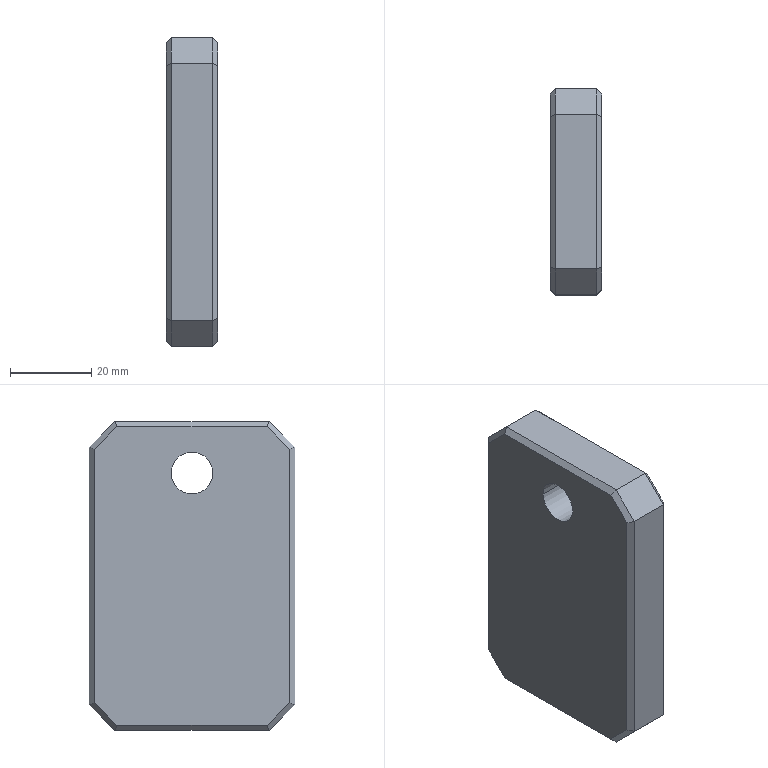Part | STEP file | 4-20.sldasm-Part-60 | 1 solid | 28 faces | box 12.7 x 50.8 x 76.2 mm | volume 46694 mm3 | plane 26 | cylinder 2 | commonest cylinder face diameters 10.317 x2
STEP:
#1=CARTESIAN_POINT('',(237.7,-154.229,175.9));
#2=VERTEX_POINT('',#1);
#3=CARTESIAN_POINT('',(237.7,-143.911,175.9));
#4=VERTEX_POINT('',#3);
#5=CARTESIAN_POINT('',(237.7,-149.07,175.9));
#6=DIRECTION('',(1.,0.,0.));
#7=DIRECTION('',(0.,0.,-1.));
#8=AXIS2_PLACEMENT_3D('',#5,#6,#7);
#9=CIRCLE('',#8,5.159);
#10=EDGE_CURVE('',#2,#4,#9,.T.);
#11=ORIENTED_EDGE('',*,*,#10,.T.);
#12=CARTESIAN_POINT('',(225.,-143.911,175.9));
#13=VERTEX_POINT('',#12);
#14=CARTESIAN_POINT('',(244.05,-143.911,175.9));
#15=DIRECTION('',(-1.,0.,0.));
#16=VECTOR('',#15,1000.);
#17=LINE('',#14,#16);
#18=EDGE_CURVE('',#4,#13,#17,.T.);
#19=ORIENTED_EDGE('',*,*,#18,.T.);
#20=CARTESIAN_POINT('',(225.,-154.229,175.9));
#21=VERTEX_POINT('',#20);
#22=CARTESIAN_POINT('',(225.,-149.07,175.9));
#23=DIRECTION('',(-1.,0.,0.));
#24=DIRECTION('',(0.,-1.,0.));
#25=AXIS2_PLACEMENT_3D('',#22,#23,#24);
#26=CIRCLE('',#25,5.159);
#27=EDGE_CURVE('',#13,#21,#26,.T.);
#28=ORIENTED_EDGE('',*,*,#27,.T.);
#29=CARTESIAN_POINT('',(244.05,-154.229,175.9));
#30=DIRECTION('',(-1.,0.,0.));
#31=VECTOR('',#30,1000.);
#32=LINE('',#29,#31);
#33=EDGE_CURVE('',#2,#21,#32,.T.);
#34=ORIENTED_EDGE('',*,*,#33,.F.);
#35=EDGE_LOOP('',(#11,#19,#28,#34));
#36=FACE_OUTER_BOUND('',#35,.T.);
#37=CARTESIAN_POINT('',(244.05,-149.07,175.9));
#38=DIRECTION('',(-1.,0.,0.));
#39=DIRECTION('',(0.,-1.,0.));
#40=AXIS2_PLACEMENT_3D('',#37,#38,#39);
#41=CYLINDRICAL_SURFACE('',#40,5.159);
#42=ADVANCED_FACE('',(#36),#41,.F.);
#43=CARTESIAN_POINT('',(237.7,-124.94,119.276));
#44=VERTEX_POINT('',#43);
#45=CARTESIAN_POINT('',(237.7,-124.94,181.724));
#46=VERTEX_POINT('',#45);
#47=CARTESIAN_POINT('',(237.7,-124.94,150.5));
#48=DIRECTION('',(0.,0.,1.));
#49=VECTOR('',#48,1000.);
#50=LINE('',#47,#49);
#51=EDGE_CURVE('',#44,#46,#50,.T.);
#52=ORIENTED_EDGE('',*,*,#51,.T.);
#53=CARTESIAN_POINT('',(237.7,-130.546,187.33));
#54=VERTEX_POINT('',#53);
#55=CARTESIAN_POINT('',(237.7,-121.393,178.177));
#56=DIRECTION('',(0.,-0.7071,0.7071));
#57=VECTOR('',#56,1000.);
#58=LINE('',#55,#57);
#59=EDGE_CURVE('',#46,#54,#58,.T.);
#60=ORIENTED_EDGE('',*,*,#59,.T.);
#61=CARTESIAN_POINT('',(237.7,-167.594,187.33));
#62=VERTEX_POINT('',#61);
#63=CARTESIAN_POINT('',(237.7,-149.07,187.33));
#64=DIRECTION('',(0.,-1.,0.));
#65=VECTOR('',#64,1000.);
#66=LINE('',#63,#65);
#67=EDGE_CURVE('',#54,#62,#66,.T.);
#68=ORIENTED_EDGE('',*,*,#67,.T.);
#69=CARTESIAN_POINT('',(237.7,-173.2,181.724));
#70=VERTEX_POINT('',#69);
#71=CARTESIAN_POINT('',(237.7,-176.747,178.177));
#72=DIRECTION('',(0.,-0.7071,-0.7071));
#73=VECTOR('',#72,1000.);
#74=LINE('',#71,#73);
#75=EDGE_CURVE('',#62,#70,#74,.T.);
#76=ORIENTED_EDGE('',*,*,#75,.T.);
#77=CARTESIAN_POINT('',(237.7,-173.2,119.276));
#78=VERTEX_POINT('',#77);
#79=CARTESIAN_POINT('',(237.7,-173.2,150.5));
#80=DIRECTION('',(0.,0.,-1.));
#81=VECTOR('',#80,1000.);
#82=LINE('',#79,#81);
#83=EDGE_CURVE('',#70,#78,#82,.T.);
#84=ORIENTED_EDGE('',*,*,#83,.T.);
#85=CARTESIAN_POINT('',(237.7,-167.594,113.67));
#86=VERTEX_POINT('',#85);
#87=CARTESIAN_POINT('',(237.7,-176.747,122.823));
#88=DIRECTION('',(0.,0.7071,-0.7071));
#89=VECTOR('',#88,1000.);
#90=LINE('',#87,#89);
#91=EDGE_CURVE('',#78,#86,#90,.T.);
#92=ORIENTED_EDGE('',*,*,#91,.T.);
#93=CARTESIAN_POINT('',(237.7,-130.546,113.67));
#94=VERTEX_POINT('',#93);
#95=CARTESIAN_POINT('',(237.7,-149.07,113.67));
#96=DIRECTION('',(0.,1.,0.));
#97=VECTOR('',#96,1000.);
#98=LINE('',#95,#97);
#99=EDGE_CURVE('',#86,#94,#98,.T.);
#100=ORIENTED_EDGE('',*,*,#99,.T.);
#101=CARTESIAN_POINT('',(237.7,-121.393,122.823));
#102=DIRECTION('',(0.,0.7071,0.7071));
#103=VECTOR('',#102,1000.);
#104=LINE('',#101,#103);
#105=EDGE_CURVE('',#94,#44,#104,.T.);
#106=ORIENTED_EDGE('',*,*,#105,.T.);
#107=EDGE_LOOP('',(#52,#60,#68,#76,#84,#92,#100,#106));
#108=FACE_OUTER_BOUND('',#107,.T.);
#109=ORIENTED_EDGE('',*,*,#10,.F.);
#110=CARTESIAN_POINT('',(237.7,-149.07,175.9));
#111=DIRECTION('',(1.,0.,0.));
#112=DIRECTION('',(0.,0.,-1.));
#113=AXIS2_PLACEMENT_3D('',#110,#111,#112);
#114=CIRCLE('',#113,5.159);
#115=EDGE_CURVE('',#4,#2,#114,.T.);
#116=ORIENTED_EDGE('',*,*,#115,.F.);
#117=EDGE_LOOP('',(#109,#116));
#118=FACE_BOUND('',#117,.T.);
#119=CARTESIAN_POINT('',(237.7,-149.07,150.5));
#120=DIRECTION('',(1.,0.,0.));
#121=DIRECTION('',(0.,1.,0.));
#122=AXIS2_PLACEMENT_3D('',#119,#120,#121);
#123=PLANE('',#122);
#124=ADVANCED_FACE('',(#108,#118),#123,.T.);
#125=CARTESIAN_POINT('',(236.43,-168.12,112.4));
#126=VERTEX_POINT('',#125);
#127=CARTESIAN_POINT('',(226.27,-168.12,112.4));
#128=VERTEX_POINT('',#127);
#129=CARTESIAN_POINT('',(225.,-168.12,112.4));
#130=DIRECTION('',(-1.,0.,0.));
#131=VECTOR('',#130,1000.);
#132=LINE('',#129,#131);
#133=EDGE_CURVE('',#126,#128,#132,.T.);
#134=ORIENTED_EDGE('',*,*,#133,.T.);
#135=CARTESIAN_POINT('',(226.27,-130.02,112.4));
#136=VERTEX_POINT('',#135);
#137=CARTESIAN_POINT('',(226.27,-149.07,112.4));
#138=DIRECTION('',(0.,1.,0.));
#139=VECTOR('',#138,1000.);
#140=LINE('',#137,#139);
#141=EDGE_CURVE('',#128,#136,#140,.T.);
#142=ORIENTED_EDGE('',*,*,#141,.T.);
#143=CARTESIAN_POINT('',(236.43,-130.02,112.4));
#144=VERTEX_POINT('',#143);
#145=CARTESIAN_POINT('',(225.,-130.02,112.4));
#146=DIRECTION('',(1.,0.,0.));
#147=VECTOR('',#146,1000.);
#148=LINE('',#145,#147);
#149=EDGE_CURVE('',#136,#144,#148,.T.);
#150=ORIENTED_EDGE('',*,*,#149,.T.);
#151=CARTESIAN_POINT('',(236.43,-149.07,112.4));
#152=DIRECTION('',(0.,-1.,0.));
#153=VECTOR('',#152,1000.);
#154=LINE('',#151,#153);
#155=EDGE_CURVE('',#144,#126,#154,.T.);
#156=ORIENTED_EDGE('',*,*,#155,.T.);
#157=EDGE_LOOP('',(#134,#142,#150,#156));
#158=FACE_OUTER_BOUND('',#157,.T.);
#159=CARTESIAN_POINT('',(225.,-149.07,112.4));
#160=DIRECTION('',(0.,0.,-1.));
#161=DIRECTION('',(-1.,0.,0.));
#162=AXIS2_PLACEMENT_3D('',#159,#160,#161);
#163=PLANE('',#162);
#164=ADVANCED_FACE('',(#158),#163,.T.);
#165=CARTESIAN_POINT('',(236.43,-174.47,182.25));
#166=VERTEX_POINT('',#165);
#167=CARTESIAN_POINT('',(226.27,-174.47,182.25));
#168=VERTEX_POINT('',#167);
#169=CARTESIAN_POINT('',(225.,-174.47,182.25));
#170=DIRECTION('',(-1.,0.,0.));
#171=VECTOR('',#170,1000.);
#172=LINE('',#169,#171);
#173=EDGE_CURVE('',#166,#168,#172,.T.);
#174=ORIENTED_EDGE('',*,*,#173,.T.);
#175=CARTESIAN_POINT('',(226.27,-174.47,118.75));
#176=VERTEX_POINT('',#175);
#177=CARTESIAN_POINT('',(226.27,-174.47,150.5));
#178=DIRECTION('',(0.,0.,-1.));
#179=VECTOR('',#178,1000.);
#180=LINE('',#177,#179);
#181=EDGE_CURVE('',#168,#176,#180,.T.);
#182=ORIENTED_EDGE('',*,*,#181,.T.);
#183=CARTESIAN_POINT('',(236.43,-174.47,118.75));
#184=VERTEX_POINT('',#183);
#185=CARTESIAN_POINT('',(225.,-174.47,118.75));
#186=DIRECTION('',(1.,0.,0.));
#187=VECTOR('',#186,1000.);
#188=LINE('',#185,#187);
#189=EDGE_CURVE('',#176,#184,#188,.T.);
#190=ORIENTED_EDGE('',*,*,#189,.T.);
#191=CARTESIAN_POINT('',(236.43,-174.47,150.5));
#192=DIRECTION('',(0.,0.,1.));
#193=VECTOR('',#192,1000.);
#194=LINE('',#191,#193);
#195=EDGE_CURVE('',#184,#166,#194,.T.);
#196=ORIENTED_EDGE('',*,*,#195,.T.);
#197=EDGE_LOOP('',(#174,#182,#190,#196));
#198=FACE_OUTER_BOUND('',#197,.T.);
#199=CARTESIAN_POINT('',(225.,-174.47,150.5));
#200=DIRECTION('',(0.,-1.,0.));
#201=DIRECTION('',(1.,0.,0.));
#202=AXIS2_PLACEMENT_3D('',#199,#200,#201);
#203=PLANE('',#202);
#204=ADVANCED_FACE('',(#198),#203,.T.);
#205=CARTESIAN_POINT('',(236.43,-130.02,188.6));
#206=VERTEX_POINT('',#205);
#207=CARTESIAN_POINT('',(226.27,-130.02,188.6));
#208=VERTEX_POINT('',#207);
#209=CARTESIAN_POINT('',(225.,-130.02,188.6));
#210=DIRECTION('',(-1.,0.,0.));
#211=VECTOR('',#210,1000.);
#212=LINE('',#209,#211);
#213=EDGE_CURVE('',#206,#208,#212,.T.);
#214=ORIENTED_EDGE('',*,*,#213,.T.);
#215=CARTESIAN_POINT('',(226.27,-168.12,188.6));
#216=VERTEX_POINT('',#215);
#217=CARTESIAN_POINT('',(226.27,-149.07,188.6));
#218=DIRECTION('',(0.,-1.,0.));
#219=VECTOR('',#218,1000.);
#220=LINE('',#217,#219);
#221=EDGE_CURVE('',#208,#216,#220,.T.);
#222=ORIENTED_EDGE('',*,*,#221,.T.);
#223=CARTESIAN_POINT('',(236.43,-168.12,188.6));
#224=VERTEX_POINT('',#223);
#225=CARTESIAN_POINT('',(225.,-168.12,188.6));
#226=DIRECTION('',(1.,0.,0.));
#227=VECTOR('',#226,1000.);
#228=LINE('',#225,#227);
#229=EDGE_CURVE('',#216,#224,#228,.T.);
#230=ORIENTED_EDGE('',*,*,#229,.T.);
#231=CARTESIAN_POINT('',(236.43,-149.07,188.6));
#232=DIRECTION('',(0.,1.,0.));
#233=VECTOR('',#232,1000.);
#234=LINE('',#231,#233);
#235=EDGE_CURVE('',#224,#206,#234,.T.);
#236=ORIENTED_EDGE('',*,*,#235,.T.);
#237=EDGE_LOOP('',(#214,#222,#230,#236));
#238=FACE_OUTER_BOUND('',#237,.T.);
#239=CARTESIAN_POINT('',(225.,-149.07,188.6));
#240=DIRECTION('',(0.,0.,1.));
#241=DIRECTION('',(1.,0.,0.));
#242=AXIS2_PLACEMENT_3D('',#239,#240,#241);
#243=PLANE('',#242);
#244=ADVANCED_FACE('',(#238),#243,.T.);
#245=CARTESIAN_POINT('',(225.,-130.546,113.67));
#246=VERTEX_POINT('',#245);
#247=CARTESIAN_POINT('',(225.,-167.594,113.67));
#248=VERTEX_POINT('',#247);
#249=CARTESIAN_POINT('',(225.,-149.07,113.67));
#250=DIRECTION('',(0.,-1.,0.));
#251=VECTOR('',#250,1000.);
#252=LINE('',#249,#251);
#253=EDGE_CURVE('',#246,#248,#252,.T.);
#254=ORIENTED_EDGE('',*,*,#253,.T.);
#255=CARTESIAN_POINT('',(225.,-173.2,119.276));
#256=VERTEX_POINT('',#255);
#257=CARTESIAN_POINT('',(225.,-176.747,122.823));
#258=DIRECTION('',(0.,-0.7071,0.7071));
#259=VECTOR('',#258,1000.);
#260=LINE('',#257,#259);
#261=EDGE_CURVE('',#248,#256,#260,.T.);
#262=ORIENTED_EDGE('',*,*,#261,.T.);
#263=CARTESIAN_POINT('',(225.,-173.2,181.724));
#264=VERTEX_POINT('',#263);
#265=CARTESIAN_POINT('',(225.,-173.2,150.5));
#266=DIRECTION('',(0.,0.,1.));
#267=VECTOR('',#266,1000.);
#268=LINE('',#265,#267);
#269=EDGE_CURVE('',#256,#264,#268,.T.);
#270=ORIENTED_EDGE('',*,*,#269,.T.);
#271=CARTESIAN_POINT('',(225.,-167.594,187.33));
#272=VERTEX_POINT('',#271);
#273=CARTESIAN_POINT('',(225.,-176.747,178.177));
#274=DIRECTION('',(0.,0.7071,0.7071));
#275=VECTOR('',#274,1000.);
#276=LINE('',#273,#275);
#277=EDGE_CURVE('',#264,#272,#276,.T.);
#278=ORIENTED_EDGE('',*,*,#277,.T.);
#279=CARTESIAN_POINT('',(225.,-130.546,187.33));
#280=VERTEX_POINT('',#279);
#281=CARTESIAN_POINT('',(225.,-149.07,187.33));
#282=DIRECTION('',(0.,1.,0.));
#283=VECTOR('',#282,1000.);
#284=LINE('',#281,#283);
#285=EDGE_CURVE('',#272,#280,#284,.T.);
#286=ORIENTED_EDGE('',*,*,#285,.T.);
#287=CARTESIAN_POINT('',(225.,-124.94,181.724));
#288=VERTEX_POINT('',#287);
#289=CARTESIAN_POINT('',(225.,-121.393,178.177));
#290=DIRECTION('',(0.,0.7071,-0.7071));
#291=VECTOR('',#290,1000.);
#292=LINE('',#289,#291);
#293=EDGE_CURVE('',#280,#288,#292,.T.);
#294=ORIENTED_EDGE('',*,*,#293,.T.);
#295=CARTESIAN_POINT('',(225.,-124.94,119.276));
#296=VERTEX_POINT('',#295);
#297=CARTESIAN_POINT('',(225.,-124.94,150.5));
#298=DIRECTION('',(0.,0.,-1.));
#299=VECTOR('',#298,1000.);
#300=LINE('',#297,#299);
#301=EDGE_CURVE('',#288,#296,#300,.T.);
#302=ORIENTED_EDGE('',*,*,#301,.T.);
#303=CARTESIAN_POINT('',(225.,-121.393,122.823));
#304=DIRECTION('',(0.,-0.7071,-0.7071));
#305=VECTOR('',#304,1000.);
#306=LINE('',#303,#305);
#307=EDGE_CURVE('',#296,#246,#306,.T.);
#308=ORIENTED_EDGE('',*,*,#307,.T.);
#309=EDGE_LOOP('',(#254,#262,#270,#278,#286,#294,#302,#308));
#310=FACE_OUTER_BOUND('',#309,.T.);
#311=CARTESIAN_POINT('',(225.,-149.07,175.9));
#312=DIRECTION('',(-1.,0.,0.));
#313=DIRECTION('',(0.,-1.,0.));
#314=AXIS2_PLACEMENT_3D('',#311,#312,#313);
#315=CIRCLE('',#314,5.159);
#316=EDGE_CURVE('',#21,#13,#315,.T.);
#317=ORIENTED_EDGE('',*,*,#316,.F.);
#318=ORIENTED_EDGE('',*,*,#27,.F.);
#319=EDGE_LOOP('',(#317,#318));
#320=FACE_BOUND('',#319,.T.);
#321=CARTESIAN_POINT('',(225.,-149.07,150.5));
#322=DIRECTION('',(-1.,0.,0.));
#323=DIRECTION('',(0.,-1.,0.));
#324=AXIS2_PLACEMENT_3D('',#321,#322,#323);
#325=PLANE('',#324);
#326=ADVANCED_FACE('',(#310,#320),#325,.T.);
#327=CARTESIAN_POINT('',(236.43,-123.67,118.75));
#328=VERTEX_POINT('',#327);
#329=CARTESIAN_POINT('',(226.27,-123.67,118.75));
#330=VERTEX_POINT('',#329);
#331=CARTESIAN_POINT('',(225.,-123.67,118.75));
#332=DIRECTION('',(-1.,0.,0.));
#333=VECTOR('',#332,1000.);
#334=LINE('',#331,#333);
#335=EDGE_CURVE('',#328,#330,#334,.T.);
#336=ORIENTED_EDGE('',*,*,#335,.T.);
#337=CARTESIAN_POINT('',(226.27,-123.67,182.25));
#338=VERTEX_POINT('',#337);
#339=CARTESIAN_POINT('',(226.27,-123.67,150.5));
#340=DIRECTION('',(0.,0.,1.));
#341=VECTOR('',#340,1000.);
#342=LINE('',#339,#341);
#343=EDGE_CURVE('',#330,#338,#342,.T.);
#344=ORIENTED_EDGE('',*,*,#343,.T.);
#345=CARTESIAN_POINT('',(236.43,-123.67,182.25));
#346=VERTEX_POINT('',#345);
#347=CARTESIAN_POINT('',(225.,-123.67,182.25));
#348=DIRECTION('',(1.,0.,0.));
#349=VECTOR('',#348,1000.);
#350=LINE('',#347,#349);
#351=EDGE_CURVE('',#338,#346,#350,.T.);
#352=ORIENTED_EDGE('',*,*,#351,.T.);
#353=CARTESIAN_POINT('',(236.43,-123.67,150.5));
#354=DIRECTION('',(0.,0.,-1.));
#355=VECTOR('',#354,1000.);
#356=LINE('',#353,#355);
#357=EDGE_CURVE('',#346,#328,#356,.T.);
#358=ORIENTED_EDGE('',*,*,#357,.T.);
#359=EDGE_LOOP('',(#336,#344,#352,#358));
#360=FACE_OUTER_BOUND('',#359,.T.);
#361=CARTESIAN_POINT('',(225.,-123.67,150.5));
#362=DIRECTION('',(0.,1.,0.));
#363=DIRECTION('',(-1.,0.,0.));
#364=AXIS2_PLACEMENT_3D('',#361,#362,#363);
#365=PLANE('',#364);
#366=ADVANCED_FACE('',(#360),#365,.T.);
#367=ORIENTED_EDGE('',*,*,#18,.F.);
#368=ORIENTED_EDGE('',*,*,#115,.T.);
#369=ORIENTED_EDGE('',*,*,#33,.T.);
#370=ORIENTED_EDGE('',*,*,#316,.T.);
#371=EDGE_LOOP('',(#367,#368,#369,#370));
#372=FACE_OUTER_BOUND('',#371,.T.);
#373=CARTESIAN_POINT('',(244.05,-149.07,175.9));
#374=DIRECTION('',(-1.,0.,0.));
#375=DIRECTION('',(0.,-1.,0.));
#376=AXIS2_PLACEMENT_3D('',#373,#374,#375);
#377=CYLINDRICAL_SURFACE('',#376,5.159);
#378=ADVANCED_FACE('',(#372),#377,.F.);
#379=ORIENTED_EDGE('',*,*,#351,.F.);
#380=CARTESIAN_POINT('',(226.27,-123.67,182.25));
#381=DIRECTION('',(0.,-0.7071,0.7071));
#382=VECTOR('',#381,1000.);
#383=LINE('',#380,#382);
#384=EDGE_CURVE('',#338,#208,#383,.T.);
#385=ORIENTED_EDGE('',*,*,#384,.T.);
#386=ORIENTED_EDGE('',*,*,#213,.F.);
#387=CARTESIAN_POINT('',(236.43,-123.67,182.25));
#388=DIRECTION('',(0.,0.7071,-0.7071));
#389=VECTOR('',#388,1000.);
#390=LINE('',#387,#389);
#391=EDGE_CURVE('',#206,#346,#390,.T.);
#392=ORIENTED_EDGE('',*,*,#391,.T.);
#393=EDGE_LOOP('',(#379,#385,#386,#392));
#394=FACE_OUTER_BOUND('',#393,.T.);
#395=CARTESIAN_POINT('',(225.,-123.67,182.25));
#396=DIRECTION('',(0.,-0.7071,-0.7071));
#397=DIRECTION('',(0.,0.7071,-0.7071));
#398=AXIS2_PLACEMENT_3D('',#395,#396,#397);
#399=PLANE('',#398);
#400=ADVANCED_FACE('',(#394),#399,.F.);
#401=ORIENTED_EDGE('',*,*,#149,.F.);
#402=CARTESIAN_POINT('',(226.27,-130.02,112.4));
#403=DIRECTION('',(0.,0.7071,0.7071));
#404=VECTOR('',#403,1000.);
#405=LINE('',#402,#404);
#406=EDGE_CURVE('',#136,#330,#405,.T.);
#407=ORIENTED_EDGE('',*,*,#406,.T.);
#408=ORIENTED_EDGE('',*,*,#335,.F.);
#409=CARTESIAN_POINT('',(236.43,-130.02,112.4));
#410=DIRECTION('',(0.,-0.7071,-0.7071));
#411=VECTOR('',#410,1000.);
#412=LINE('',#409,#411);
#413=EDGE_CURVE('',#328,#144,#412,.T.);
#414=ORIENTED_EDGE('',*,*,#413,.T.);
#415=EDGE_LOOP('',(#401,#407,#408,#414));
#416=FACE_OUTER_BOUND('',#415,.T.);
#417=CARTESIAN_POINT('',(225.,-130.02,112.4));
#418=DIRECTION('',(0.,-0.7071,0.7071));
#419=DIRECTION('',(0.,-0.7071,-0.7071));
#420=AXIS2_PLACEMENT_3D('',#417,#418,#419);
#421=PLANE('',#420);
#422=ADVANCED_FACE('',(#416),#421,.F.);
#423=ORIENTED_EDGE('',*,*,#189,.F.);
#424=CARTESIAN_POINT('',(226.27,-174.47,118.75));
#425=DIRECTION('',(0.,0.7071,-0.7071));
#426=VECTOR('',#425,1000.);
#427=LINE('',#424,#426);
#428=EDGE_CURVE('',#176,#128,#427,.T.);
#429=ORIENTED_EDGE('',*,*,#428,.T.);
#430=ORIENTED_EDGE('',*,*,#133,.F.);
#431=CARTESIAN_POINT('',(236.43,-174.47,118.75));
#432=DIRECTION('',(0.,-0.7071,0.7071));
#433=VECTOR('',#432,1000.);
#434=LINE('',#431,#433);
#435=EDGE_CURVE('',#126,#184,#434,.T.);
#436=ORIENTED_EDGE('',*,*,#435,.T.);
#437=EDGE_LOOP('',(#423,#429,#430,#436));
#438=FACE_OUTER_BOUND('',#437,.T.);
#439=CARTESIAN_POINT('',(225.,-174.47,118.75));
#440=DIRECTION('',(0.,0.7071,0.7071));
#441=DIRECTION('',(0.,-0.7071,0.7071));
#442=AXIS2_PLACEMENT_3D('',#439,#440,#441);
#443=PLANE('',#442);
#444=ADVANCED_FACE('',(#438),#443,.F.);
#445=ORIENTED_EDGE('',*,*,#229,.F.);
#446=CARTESIAN_POINT('',(226.27,-168.12,188.6));
#447=DIRECTION('',(0.,-0.7071,-0.7071));
#448=VECTOR('',#447,1000.);
#449=LINE('',#446,#448);
#450=EDGE_CURVE('',#216,#168,#449,.T.);
#451=ORIENTED_EDGE('',*,*,#450,.T.);
#452=ORIENTED_EDGE('',*,*,#173,.F.);
#453=CARTESIAN_POINT('',(236.43,-168.12,188.6));
#454=DIRECTION('',(0.,0.7071,0.7071));
#455=VECTOR('',#454,1000.);
#456=LINE('',#453,#455);
#457=EDGE_CURVE('',#166,#224,#456,.T.);
#458=ORIENTED_EDGE('',*,*,#457,.T.);
#459=EDGE_LOOP('',(#445,#451,#452,#458));
#460=FACE_OUTER_BOUND('',#459,.T.);
#461=CARTESIAN_POINT('',(225.,-168.12,188.6));
#462=DIRECTION('',(0.,0.7071,-0.7071));
#463=DIRECTION('',(0.,0.7071,0.7071));
#464=AXIS2_PLACEMENT_3D('',#461,#462,#463);
#465=PLANE('',#464);
#466=ADVANCED_FACE('',(#460),#465,.F.);
#467=CARTESIAN_POINT('',(222.636,-131.525,184.966));
#468=DIRECTION('',(-0.6786,-0.2811,-0.6786));
#469=VECTOR('',#468,1000.);
#470=LINE('',#467,#469);
#471=EDGE_CURVE('',#208,#280,#470,.T.);
#472=ORIENTED_EDGE('',*,*,#471,.F.);
#473=ORIENTED_EDGE('',*,*,#384,.F.);
#474=CARTESIAN_POINT('',(225.957,-123.983,182.12));
#475=DIRECTION('',(0.6786,0.6786,0.2811));
#476=VECTOR('',#475,1000.);
#477=LINE('',#474,#476);
#478=EDGE_CURVE('',#288,#338,#477,.T.);
#479=ORIENTED_EDGE('',*,*,#478,.F.);
#480=ORIENTED_EDGE('',*,*,#293,.F.);
#481=EDGE_LOOP('',(#472,#473,#479,#480));
#482=FACE_OUTER_BOUND('',#481,.T.);
#483=CARTESIAN_POINT('',(225.,-121.393,178.177));
#484=DIRECTION('',(-0.7071,0.5,0.5));
#485=DIRECTION('',(-0.5774,-0.8165,0.));
#486=AXIS2_PLACEMENT_3D('',#483,#484,#485);
#487=PLANE('',#486);
#488=ADVANCED_FACE('',(#482),#487,.T.);
#489=ORIENTED_EDGE('',*,*,#478,.T.);
#490=ORIENTED_EDGE('',*,*,#343,.F.);
#491=CARTESIAN_POINT('',(220.214,-129.726,121.259));
#492=DIRECTION('',(0.6786,0.6786,-0.2811));
#493=VECTOR('',#492,1000.);
#494=LINE('',#491,#493);
#495=EDGE_CURVE('',#296,#330,#494,.T.);
#496=ORIENTED_EDGE('',*,*,#495,.F.);
#497=ORIENTED_EDGE('',*,*,#301,.F.);
#498=EDGE_LOOP('',(#489,#490,#496,#497));
#499=FACE_OUTER_BOUND('',#498,.T.);
#500=CARTESIAN_POINT('',(226.27,-123.67,150.5));
#501=DIRECTION('',(0.7071,-0.7071,0.));
#502=DIRECTION('',(0.7071,0.7071,0.));
#503=AXIS2_PLACEMENT_3D('',#500,#501,#502);
#504=PLANE('',#503);
#505=ADVANCED_FACE('',(#499),#504,.F.);
#506=ORIENTED_EDGE('',*,*,#471,.T.);
#507=ORIENTED_EDGE('',*,*,#285,.F.);
#508=CARTESIAN_POINT('',(222.531,-166.571,184.861));
#509=DIRECTION('',(-0.6786,0.2811,-0.6786));
#510=VECTOR('',#509,1000.);
#511=LINE('',#508,#510);
#512=EDGE_CURVE('',#216,#272,#511,.T.);
#513=ORIENTED_EDGE('',*,*,#512,.F.);
#514=ORIENTED_EDGE('',*,*,#221,.F.);
#515=EDGE_LOOP('',(#506,#507,#513,#514));
#516=FACE_OUTER_BOUND('',#515,.T.);
#517=CARTESIAN_POINT('',(226.27,-149.07,188.6));
#518=DIRECTION('',(0.7071,0.,-0.7071));
#519=DIRECTION('',(-0.7071,0.,-0.7071));
#520=AXIS2_PLACEMENT_3D('',#517,#518,#519);
#521=PLANE('',#520);
#522=ADVANCED_FACE('',(#516),#521,.F.);
#523=ORIENTED_EDGE('',*,*,#495,.T.);
#524=ORIENTED_EDGE('',*,*,#406,.F.);
#525=CARTESIAN_POINT('',(222.531,-131.569,116.139));
#526=DIRECTION('',(0.6786,0.2811,-0.6786));
#527=VECTOR('',#526,1000.);
#528=LINE('',#525,#527);
#529=EDGE_CURVE('',#246,#136,#528,.T.);
#530=ORIENTED_EDGE('',*,*,#529,.F.);
#531=ORIENTED_EDGE('',*,*,#307,.F.);
#532=EDGE_LOOP('',(#523,#524,#530,#531));
#533=FACE_OUTER_BOUND('',#532,.T.);
#534=CARTESIAN_POINT('',(225.,-121.393,122.823));
#535=DIRECTION('',(-0.7071,0.5,-0.5));
#536=DIRECTION('',(-0.5774,0.,0.8165));
#537=AXIS2_PLACEMENT_3D('',#534,#535,#536);
#538=PLANE('',#537);
#539=ADVANCED_FACE('',(#533),#538,.T.);
#540=ORIENTED_EDGE('',*,*,#512,.T.);
#541=ORIENTED_EDGE('',*,*,#277,.F.);
#542=CARTESIAN_POINT('',(225.957,-174.157,182.12));
#543=DIRECTION('',(-0.6786,0.6786,-0.2811));
#544=VECTOR('',#543,1000.);
#545=LINE('',#542,#544);
#546=EDGE_CURVE('',#168,#264,#545,.T.);
#547=ORIENTED_EDGE('',*,*,#546,.F.);
#548=ORIENTED_EDGE('',*,*,#450,.F.);
#549=EDGE_LOOP('',(#540,#541,#547,#548));
#550=FACE_OUTER_BOUND('',#549,.T.);
#551=CARTESIAN_POINT('',(225.,-176.747,178.177));
#552=DIRECTION('',(-0.7071,-0.5,0.5));
#553=DIRECTION('',(0.5774,-0.8165,0.));
#554=AXIS2_PLACEMENT_3D('',#551,#552,#553);
#555=PLANE('',#554);
#556=ADVANCED_FACE('',(#550),#555,.T.);
#557=ORIENTED_EDGE('',*,*,#529,.T.);
#558=ORIENTED_EDGE('',*,*,#141,.F.);
#559=CARTESIAN_POINT('',(222.636,-166.615,116.034));
#560=DIRECTION('',(0.6786,-0.2811,-0.6786));
#561=VECTOR('',#560,1000.);
#562=LINE('',#559,#561);
#563=EDGE_CURVE('',#248,#128,#562,.T.);
#564=ORIENTED_EDGE('',*,*,#563,.F.);
#565=ORIENTED_EDGE('',*,*,#253,.F.);
#566=EDGE_LOOP('',(#557,#558,#564,#565));
#567=FACE_OUTER_BOUND('',#566,.T.);
#568=CARTESIAN_POINT('',(226.27,-149.07,112.4));
#569=DIRECTION('',(0.7071,0.,0.7071));
#570=DIRECTION('',(0.7071,0.,-0.7071));
#571=AXIS2_PLACEMENT_3D('',#568,#569,#570);
#572=PLANE('',#571);
#573=ADVANCED_FACE('',(#567),#572,.F.);
#574=ORIENTED_EDGE('',*,*,#546,.T.);
#575=ORIENTED_EDGE('',*,*,#269,.F.);
#576=CARTESIAN_POINT('',(220.214,-168.414,121.259));
#577=DIRECTION('',(-0.6786,0.6786,0.2811));
#578=VECTOR('',#577,1000.);
#579=LINE('',#576,#578);
#580=EDGE_CURVE('',#176,#256,#579,.T.);
#581=ORIENTED_EDGE('',*,*,#580,.F.);
#582=ORIENTED_EDGE('',*,*,#181,.F.);
#583=EDGE_LOOP('',(#574,#575,#581,#582));
#584=FACE_OUTER_BOUND('',#583,.T.);
#585=CARTESIAN_POINT('',(226.27,-174.47,150.5));
#586=DIRECTION('',(0.7071,0.7071,0.));
#587=DIRECTION('',(-0.7071,0.7071,0.));
#588=AXIS2_PLACEMENT_3D('',#585,#586,#587);
#589=PLANE('',#588);
#590=ADVANCED_FACE('',(#584),#589,.F.);
#591=ORIENTED_EDGE('',*,*,#563,.T.);
#592=ORIENTED_EDGE('',*,*,#428,.F.);
#593=ORIENTED_EDGE('',*,*,#580,.T.);
#594=ORIENTED_EDGE('',*,*,#261,.F.);
#595=EDGE_LOOP('',(#591,#592,#593,#594));
#596=FACE_OUTER_BOUND('',#595,.T.);
#597=CARTESIAN_POINT('',(225.,-176.747,122.823));
#598=DIRECTION('',(-0.7071,-0.5,-0.5));
#599=DIRECTION('',(-0.5774,0.,0.8165));
#600=AXIS2_PLACEMENT_3D('',#597,#598,#599);
#601=PLANE('',#600);
#602=ADVANCED_FACE('',(#596),#601,.T.);
#603=CARTESIAN_POINT('',(242.486,-168.414,121.259));
#604=DIRECTION('',(0.6786,0.6786,0.2811));
#605=VECTOR('',#604,1000.);
#606=LINE('',#603,#605);
#607=EDGE_CURVE('',#184,#78,#606,.T.);
#608=ORIENTED_EDGE('',*,*,#607,.F.);
#609=ORIENTED_EDGE('',*,*,#435,.F.);
#610=CARTESIAN_POINT('',(240.169,-166.571,116.139));
#611=DIRECTION('',(-0.6786,-0.2811,-0.6786));
#612=VECTOR('',#611,1000.);
#613=LINE('',#610,#612);
#614=EDGE_CURVE('',#86,#126,#613,.T.);
#615=ORIENTED_EDGE('',*,*,#614,.F.);
#616=ORIENTED_EDGE('',*,*,#91,.F.);
#617=EDGE_LOOP('',(#608,#609,#615,#616));
#618=FACE_OUTER_BOUND('',#617,.T.);
#619=CARTESIAN_POINT('',(237.7,-176.747,122.823));
#620=DIRECTION('',(0.7071,-0.5,-0.5));
#621=DIRECTION('',(-0.5774,0.,-0.8165));
#622=AXIS2_PLACEMENT_3D('',#619,#620,#621);
#623=PLANE('',#622);
#624=ADVANCED_FACE('',(#618),#623,.T.);
#625=ORIENTED_EDGE('',*,*,#614,.T.);
#626=ORIENTED_EDGE('',*,*,#155,.F.);
#627=CARTESIAN_POINT('',(240.064,-131.525,116.034));
#628=DIRECTION('',(-0.6786,0.2811,-0.6786));
#629=VECTOR('',#628,1000.);
#630=LINE('',#627,#629);
#631=EDGE_CURVE('',#94,#144,#630,.T.);
#632=ORIENTED_EDGE('',*,*,#631,.F.);
#633=ORIENTED_EDGE('',*,*,#99,.F.);
#634=EDGE_LOOP('',(#625,#626,#632,#633));
#635=FACE_OUTER_BOUND('',#634,.T.);
#636=CARTESIAN_POINT('',(236.43,-149.07,112.4));
#637=DIRECTION('',(-0.7071,0.,0.7071));
#638=DIRECTION('',(0.7071,0.,0.7071));
#639=AXIS2_PLACEMENT_3D('',#636,#637,#638);
#640=PLANE('',#639);
#641=ADVANCED_FACE('',(#635),#640,.F.);
#642=ORIENTED_EDGE('',*,*,#607,.T.);
#643=ORIENTED_EDGE('',*,*,#83,.F.);
#644=CARTESIAN_POINT('',(236.743,-174.157,182.12));
#645=DIRECTION('',(0.6786,0.6786,-0.2811));
#646=VECTOR('',#645,1000.);
#647=LINE('',#644,#646);
#648=EDGE_CURVE('',#166,#70,#647,.T.);
#649=ORIENTED_EDGE('',*,*,#648,.F.);
#650=ORIENTED_EDGE('',*,*,#195,.F.);
#651=EDGE_LOOP('',(#642,#643,#649,#650));
#652=FACE_OUTER_BOUND('',#651,.T.);
#653=CARTESIAN_POINT('',(236.43,-174.47,150.5));
#654=DIRECTION('',(-0.7071,0.7071,0.));
#655=DIRECTION('',(-0.7071,-0.7071,0.));
#656=AXIS2_PLACEMENT_3D('',#653,#654,#655);
#657=PLANE('',#656);
#658=ADVANCED_FACE('',(#652),#657,.F.);
#659=ORIENTED_EDGE('',*,*,#631,.T.);
#660=ORIENTED_EDGE('',*,*,#413,.F.);
#661=CARTESIAN_POINT('',(236.743,-123.983,118.88));
#662=DIRECTION('',(-0.6786,0.6786,-0.2811));
#663=VECTOR('',#662,1000.);
#664=LINE('',#661,#663);
#665=EDGE_CURVE('',#44,#328,#664,.T.);
#666=ORIENTED_EDGE('',*,*,#665,.F.);
#667=ORIENTED_EDGE('',*,*,#105,.F.);
#668=EDGE_LOOP('',(#659,#660,#666,#667));
#669=FACE_OUTER_BOUND('',#668,.T.);
#670=CARTESIAN_POINT('',(237.7,-121.393,122.823));
#671=DIRECTION('',(0.7071,0.5,-0.5));
#672=DIRECTION('',(-0.5774,0.,-0.8165));
#673=AXIS2_PLACEMENT_3D('',#670,#671,#672);
#674=PLANE('',#673);
#675=ADVANCED_FACE('',(#669),#674,.T.);
#676=ORIENTED_EDGE('',*,*,#648,.T.);
#677=ORIENTED_EDGE('',*,*,#75,.F.);
#678=CARTESIAN_POINT('',(240.169,-166.571,184.861));
#679=DIRECTION('',(0.6786,0.2811,-0.6786));
#680=VECTOR('',#679,1000.);
#681=LINE('',#678,#680);
#682=EDGE_CURVE('',#224,#62,#681,.T.);
#683=ORIENTED_EDGE('',*,*,#682,.F.);
#684=ORIENTED_EDGE('',*,*,#457,.F.);
#685=EDGE_LOOP('',(#676,#677,#683,#684));
#686=FACE_OUTER_BOUND('',#685,.T.);
#687=CARTESIAN_POINT('',(237.7,-176.747,178.177));
#688=DIRECTION('',(0.7071,-0.5,0.5));
#689=DIRECTION('',(0.5774,0.8165,0.));
#690=AXIS2_PLACEMENT_3D('',#687,#688,#689);
#691=PLANE('',#690);
#692=ADVANCED_FACE('',(#686),#691,.T.);
#693=ORIENTED_EDGE('',*,*,#665,.T.);
#694=ORIENTED_EDGE('',*,*,#357,.F.);
#695=CARTESIAN_POINT('',(242.486,-129.726,179.741));
#696=DIRECTION('',(-0.6786,0.6786,0.2811));
#697=VECTOR('',#696,1000.);
#698=LINE('',#695,#697);
#699=EDGE_CURVE('',#46,#346,#698,.T.);
#700=ORIENTED_EDGE('',*,*,#699,.F.);
#701=ORIENTED_EDGE('',*,*,#51,.F.);
#702=EDGE_LOOP('',(#693,#694,#700,#701));
#703=FACE_OUTER_BOUND('',#702,.T.);
#704=CARTESIAN_POINT('',(236.43,-123.67,150.5));
#705=DIRECTION('',(-0.7071,-0.7071,0.));
#706=DIRECTION('',(0.7071,-0.7071,0.));
#707=AXIS2_PLACEMENT_3D('',#704,#705,#706);
#708=PLANE('',#707);
#709=ADVANCED_FACE('',(#703),#708,.F.);
#710=ORIENTED_EDGE('',*,*,#682,.T.);
#711=ORIENTED_EDGE('',*,*,#67,.F.);
#712=CARTESIAN_POINT('',(240.064,-131.525,184.966));
#713=DIRECTION('',(0.6786,-0.2811,-0.6786));
#714=VECTOR('',#713,1000.);
#715=LINE('',#712,#714);
#716=EDGE_CURVE('',#206,#54,#715,.T.);
#717=ORIENTED_EDGE('',*,*,#716,.F.);
#718=ORIENTED_EDGE('',*,*,#235,.F.);
#719=EDGE_LOOP('',(#710,#711,#717,#718));
#720=FACE_OUTER_BOUND('',#719,.T.);
#721=CARTESIAN_POINT('',(236.43,-149.07,188.6));
#722=DIRECTION('',(-0.7071,0.,-0.7071));
#723=DIRECTION('',(-0.7071,0.,0.7071));
#724=AXIS2_PLACEMENT_3D('',#721,#722,#723);
#725=PLANE('',#724);
#726=ADVANCED_FACE('',(#720),#725,.F.);
#727=ORIENTED_EDGE('',*,*,#699,.T.);
#728=ORIENTED_EDGE('',*,*,#391,.F.);
#729=ORIENTED_EDGE('',*,*,#716,.T.);
#730=ORIENTED_EDGE('',*,*,#59,.F.);
#731=EDGE_LOOP('',(#727,#728,#729,#730));
#732=FACE_OUTER_BOUND('',#731,.T.);
#733=CARTESIAN_POINT('',(237.7,-121.393,178.177));
#734=DIRECTION('',(0.7071,0.5,0.5));
#735=DIRECTION('',(-0.5774,0.8165,0.));
#736=AXIS2_PLACEMENT_3D('',#733,#734,#735);
#737=PLANE('',#736);
#738=ADVANCED_FACE('',(#732),#737,.T.);
#739=CLOSED_SHELL('',(#42,#124,#164,#204,#244,#326,#366,#378,#400,#422,#444,#466,#488,#505,#522,#539,#556,#573,#590,#602,#624,#641,#658,#675,#692,#709,#726,#738));
#740=MANIFOLD_SOLID_BREP('',#739);
#741=CARTESIAN_POINT('',(0.,0.,0.));
#742=DIRECTION('',(0.,0.,1.));
#743=DIRECTION('',(1.,0.,0.));
#744=AXIS2_PLACEMENT_3D('',#741,#742,#743);
#745=(LENGTH_UNIT()NAMED_UNIT(*)SI_UNIT(.MILLI.,.METRE.));
#746=UNCERTAINTY_MEASURE_WITH_UNIT(LENGTH_MEASURE(0.00001),#745,'','');
#747=(NAMED_UNIT(*)PLANE_ANGLE_UNIT()SI_UNIT($,.RADIAN.));
#748=(NAMED_UNIT(*)SI_UNIT($,.STERADIAN.)SOLID_ANGLE_UNIT());
#749=(GEOMETRIC_REPRESENTATION_CONTEXT(3)GLOBAL_UNCERTAINTY_ASSIGNED_CONTEXT((#746))GLOBAL_UNIT_ASSIGNED_CONTEXT((#745,#747,#748))REPRESENTATION_CONTEXT('',''));
#750=ADVANCED_BREP_SHAPE_REPRESENTATION('',(#740,#744),#749);